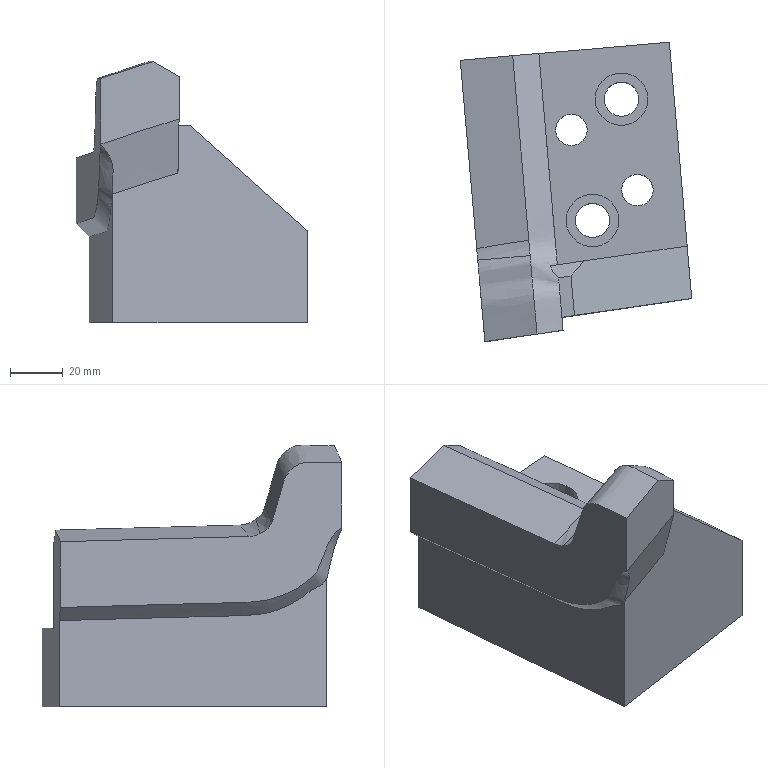Part | NX | features solid 2 | 1 solid | 28 faces | box 88.025 x 114.036 x 99.61 mm | volume 362150 mm3 | spline 12 | plane 10 | cylinder 6 | commonest cylinder face diameters 12 x2 13 x2 20 x2